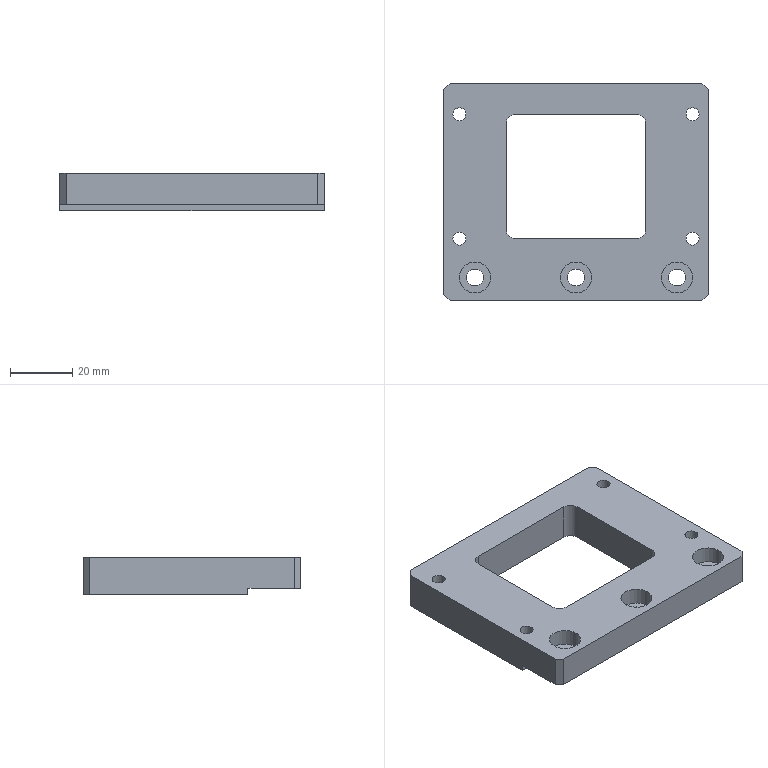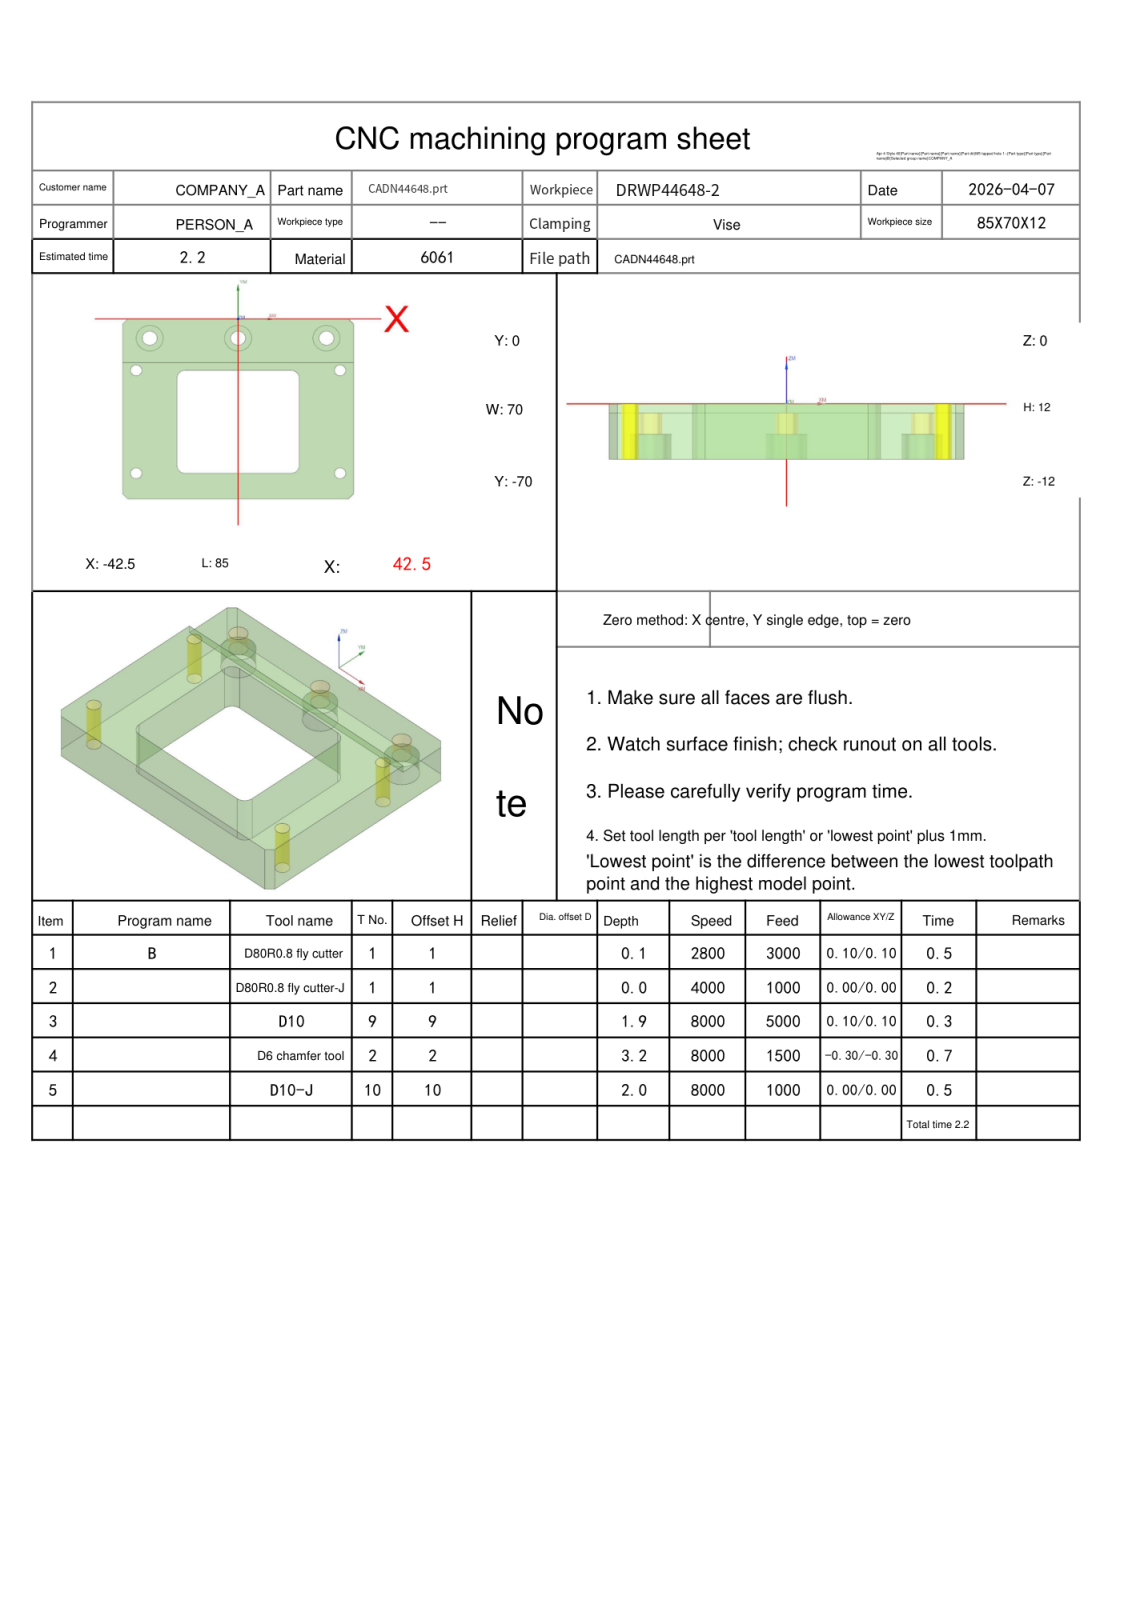NC program | NX | posted by the shop | part box 85 x 70 x 12 mm
Whole program:
%
O0001
(Machine time: 3.09 MIN)
(===Total Tool:4===)
(T1=D80R0.8 fly cutter D=80.  R=0.8  D-  H01 Z=0.    )
(T9=D10     D=10.  R=0.   D-  H09 Z=-1.9  )
(T2=D6 chamfer tool   D=6.   R=0.   D-  H02 Z=-3.2  )
(T10=D10-J  D=10.  R=0.   D10 H10 Z=-2.   )
G80 G90 G17 G49 G40
G91 G28 Z0
M01
N1 T01 M06
(D80R0.8 fly cutter  D=80. R=0.8 H=01 ce=0.10 di=0.10)
G00 G90 G54 X94.597 Y-35. M03 S2800
G43 H01 Z20.
M08
Z4.517
G01 Z2.517 F3000.
X82.597
X-82.597
X-94.597
Z4.517
G00 X94.597
Z4.033
G01 Z2.033
X82.597
X-82.597
X-94.597
Z4.033
G00 X94.597
Z3.55
G01 Z1.55
X82.597
X-82.597
X-94.597
Z3.55
G00 X94.597
Z3.067
G01 Z1.067
X82.597
X-82.597
X-94.597
Z3.067
G00 Z20.
X94.597
Z2.583
G01 Z.583
X82.597
X-82.597
X-94.597
Z2.583
G00 Z20.
X94.597
Z2.1
G01 Z.1
X82.597
X-82.597
X-94.597
Z2.1
G00 Z20.
G91 G28 Z0.0
M05
M09
G91 G28 Z0.0
M01
N2 T01 M06
(D80R0.8 fly cutter-J  D=80. R=0.8 H=01 ce=0.00 di=0.00)
G00 G90 G54 X94.499 Y-35. M03 S4000
G43 H01 Z20.
M08
Z2.
G01 Z0.0 F1000.
X82.499
X-82.499
X-94.499
Z2.
G00 Z20.
G91 G28 Z0.0
M05
M09
G91 G28 Z0.0
M01
N3 T09 M06
(D10  D=10. R=0. H=09 ce=0.10 di=0.10)
G00 G90 G54 X-48.714 Y3.1 M03 S8000
G43 H09 Z12.8
M08
Z1.025
G01 Z-.475 F5000.
X-44.33
X43.916
G02 X44.622 Y2.808 I-.001 J-1.
G01 X47.107 Y.322
G02 X47.4 Y-.384 I-.707 J-.707
G01 Y-3.401
G02 X46.401 Y-4.4 I-1. J.001
G01 X-46.544
G03 X-47.532 Y-5.245 I.001 J-1.
G01 X-48.388 Y-10.746
X-48.4 Y-10.9
G03 X-47.4 Y-11.9 I1. J0.0
G01 X47.4
X50.6
Z1.025
G00 X-48.714 Y3.1
Z.55
G01 Z-.95
X-44.33
X43.916
G02 X44.622 Y2.808 I-.001 J-1.
G01 X47.107 Y.322
G02 X47.4 Y-.384 I-.707 J-.707
G01 Y-3.401
G02 X46.401 Y-4.4 I-1. J.001
G01 X-46.544
G03 X-47.532 Y-5.245 I.001 J-1.
G01 X-48.388 Y-10.746
X-48.4 Y-10.9
G03 X-47.4 Y-11.9 I1. J0.0
G01 X47.4
X50.6
Z.55
G00 X-48.714 Y3.1
Z.075
G01 Z-1.425
X-44.33
X43.916
G02 X44.622 Y2.808 I-.001 J-1.
G01 X47.107 Y.322
G02 X47.4 Y-.384 I-.707 J-.707
G01 Y-3.401
G02 X46.401 Y-4.4 I-1. J.001
G01 X-46.544
G03 X-47.532 Y-5.245 I.001 J-1.
G01 X-48.388 Y-10.746
X-48.4 Y-10.9
G03 X-47.4 Y-11.9 I1. J0.0
G01 X47.4
X50.6
Z.075
G00 X-48.714 Y3.1
Z-.4
G01 Z-1.9
X-44.33
X43.916
G02 X44.622 Y2.808 I-.001 J-1.
G01 X47.107 Y.322
G02 X47.4 Y-.384 I-.707 J-.707
G01 Y-3.401
G02 X46.401 Y-4.4 I-1. J.001
G01 X-46.544
G03 X-47.532 Y-5.245 I.001 J-1.
G01 X-48.388 Y-10.746
X-48.4 Y-10.9
G03 X-47.4 Y-11.9 I1. J0.0
G01 X47.4
X50.6
Z-.4
G00 Z12.8
G91 G28 Z0.0
M05
M09
G91 G28 Z0.0
M01
N4 T02 M06
(D6 chamfer tool  D=6. R=0. H=02 ce=0.00 di=0.10)
G00 G90 G54 X-37.5 Y-20. M03 S8000
G43 H02 Z20.
M08
G98 G81 X-37.5 Y-20. Z-2.7 R3. F1000.
Y-60.
X37.5
Y-20.
G80
G00 Z20.
G00 G90 X-13.499 Y-20.7 M03 S7000
Z20.
Z2.5
G01 X-19.618 Z.273 F1500.
X-19.923 Y-20.736 Z.161
X-20.22 Y-20.813 Z.049
X-20.505 Y-20.928 Z-.063
X-20.772 Y-21.08 Z-.174
X-21.016 Y-21.267 Z-.286
X-21.233 Y-21.484 Z-.398
X-21.42 Y-21.728 Z-.51
X-21.572 Y-21.995 Z-.622
X-21.687 Y-22.28 Z-.734
X-21.764 Y-22.577 Z-.845
X-21.8 Y-22.882 Z-.957
Y-23. Z-1.
Y-57.
G03 X-19.5 Y-59.3 I2.3 J0.0
G01 X19.5
G03 X21.8 Y-57. I0.0 J2.3
G01 Y-23.
G03 X19.5 Y-20.7 I-2.3 J0.0
G01 X-19.5
G03 X-21.8 Y-23. I0.0 J-2.3
G01 Y-23.5
Z1.5
G00 Z20.
G00 G90 X-.386 Y-15.773 M03 S6500
Z20.
Z.172
G01 Z-1.2 F1500.
G03 X-.1 Y-15.973 I1.286 J1.532
G01 X-.054 Y-16.003
X0.0 Y-16.
X42.5
G02 X43.5 Y-17. I0.0 J-1.
G01 Y-68.
X43.466 Y-68.259
X43.366 Y-68.5
X43.207 Y-68.707
X41.207 Y-70.707
X41. Y-70.866
X40.759 Y-70.966
X40.5 Y-71.
X-40.5
X-40.759 Y-70.966
X-41. Y-70.866
X-41.207 Y-70.707
X-43.207 Y-68.707
X-43.366 Y-68.5
X-43.466 Y-68.259
X-43.5 Y-68.
Y-17.
G02 X-42.5 Y-16. I1. J0.0
G01 X0.0
X.054 Y-16.003
X.1 Y-15.973
G03 X.386 Y-15.773 I-1. J1.732
G01 Z.172
G00 Z10.
X-38.426 Y-19.588
Z.32
G01 Z-1.2
G03 X-38.586 Y-19.897 I1.687 J-1.075
G01 X-38.61 Y-19.946
X-38.6 Y-20.
G03 X-37.5 Y-21.1 I1.1 J0.0
X-36.4 Y-20. I0.0 J1.1
X-37.5 Y-18.9 I-1.1 J0.0
X-38.6 Y-20. I0.0 J-1.1
G01 X-38.61 Y-20.054
X-38.586 Y-20.103
G03 X-38.426 Y-20.412 I1.848 J.765
G01 Z.32
G00 Z10.
Y-59.588
Z.32
G01 Z-1.2
G03 X-38.586 Y-59.897 I1.687 J-1.075
G01 X-38.61 Y-59.946
X-38.6 Y-60.
G03 X-37.5 Y-61.1 I1.1 J0.0
X-36.4 Y-60. I0.0 J1.1
X-37.5 Y-58.9 I-1.1 J0.0
X-38.6 Y-60. I0.0 J-1.1
G01 X-38.61 Y-60.054
X-38.586 Y-60.103
G03 X-38.426 Y-60.412 I1.848 J.765
G01 Z.32
G00 Z10.
X21.273 Y-40.386
Z.172
G01 Z-1.2
G03 X21.473 Y-40.1 I-1.532 J1.286
G01 X21.503 Y-40.054
X21.5 Y-40.
Y-23.
G03 X19.5 Y-21. I-2. J0.0
G01 X-19.5
G03 X-21.5 Y-23. I0.0 J-2.
G01 Y-57.
G03 X-19.5 Y-59. I2. J0.0
G01 X19.5
G03 X21.5 Y-57. I0.0 J2.
G01 Y-40.
X21.503 Y-39.946
X21.473 Y-39.9
G03 X21.273 Y-39.614 I-1.732 J-1.
G01 Z.172
G00 Z10.
X36.574 Y-59.588
Z.32
G01 Z-1.2
G03 X36.414 Y-59.897 I1.687 J-1.075
G01 X36.39 Y-59.946
X36.4 Y-60.
G03 X37.5 Y-61.1 I1.1 J0.0
X38.6 Y-60. I0.0 J1.1
X37.5 Y-58.9 I-1.1 J0.0
X36.4 Y-60. I0.0 J-1.1
G01 X36.39 Y-60.054
X36.414 Y-60.103
G03 X36.574 Y-60.412 I1.848 J.765
G01 Z.32
G00 Z10.
Y-19.588
Z.32
G01 Z-1.2
G03 X36.414 Y-19.897 I1.687 J-1.075
G01 X36.39 Y-19.946
X36.4 Y-20.
G03 X37.5 Y-21.1 I1.1 J0.0
X38.6 Y-20. I0.0 J1.1
X37.5 Y-18.9 I-1.1 J0.0
X36.4 Y-20. I0.0 J-1.1
G01 X36.39 Y-20.054
X36.414 Y-20.103
G03 X36.574 Y-20.412 I1.848 J.765
G01 Z.32
G00 Z10.
X-43.568 Y-14.01
Z-1.669
G01 Z-3.2
X-43.508 Y-13.925
X-43.5 Y-13.895
Y-2.
X-43.466 Y-1.741
X-43.366 Y-1.5
X-43.207 Y-1.293
X-41.207 Y.707
X-41. Y.866
X-40.759 Y.966
X-40.5 Y1.
X40.5
X40.759 Y.966
X41. Y.866
X41.207 Y.707
X43.207 Y-1.293
X43.366 Y-1.5
X43.466 Y-1.741
X43.5 Y-2.
Y-13.895
X43.508 Y-13.925
X43.568 Y-14.01
Z-1.669
G00 Z10.
X30.935 Y-7.093
Z-1.73
G01 Z-3.2
G03 X30.766 Y-7.398 I1.658 J-1.118
G01 X30.741 Y-7.446
X30.75 Y-7.5
G03 X32.5 Y-9.25 I1.75 J0.0
X34.25 Y-7.5 I0.0 J1.75
X32.5 Y-5.75 I-1.75 J0.0
X30.75 Y-7.5 I0.0 J-1.75
G01 X30.741 Y-7.554
X30.766 Y-7.602
G03 X30.935 Y-7.907 I1.827 J.813
G01 Z-1.73
G00 Z10.
X-1.565 Y-7.093
Z-1.73
G01 Z-3.2
G03 X-1.734 Y-7.398 I1.658 J-1.118
G01 X-1.759 Y-7.446
X-1.75 Y-7.5
G03 X0.0 Y-9.25 I1.75 J0.0
X1.75 Y-7.5 I0.0 J1.75
X0.0 Y-5.75 I-1.75 J0.0
X-1.75 Y-7.5 I0.0 J-1.75
G01 X-1.759 Y-7.554
X-1.734 Y-7.602
G03 X-1.565 Y-7.907 I1.827 J.813
G01 Z-1.73
G00 Z10.
X-34.065 Y-7.093
Z-1.73
G01 Z-3.2
G03 X-34.234 Y-7.398 I1.658 J-1.118
G01 X-34.259 Y-7.446
X-34.25 Y-7.5
G03 X-32.5 Y-9.25 I1.75 J0.0
X-30.75 Y-7.5 I0.0 J1.75
X-32.5 Y-5.75 I-1.75 J0.0
X-34.25 Y-7.5 I0.0 J-1.75
G01 X-34.259 Y-7.554
X-34.234 Y-7.602
G03 X-34.065 Y-7.907 I1.827 J.813
G01 Z-1.73
G00 Z20.
G91 G28 Z0.0
M05
M09
G91 G28 Z0.0
M01
N5 T10 M06
(D10-J  D=10. R=0. H=10 ce=0.40 di=0.00)
G00 G90 G54 X-48.337 Y2.062 M03 S8000
G43 H10 Z12.8
M08
Z-.5
G01 Z-2. F1000.
G03 X-46.571 Y1. I1.766 J.938
G01 X46.158
G02 X46.863 Y.708 I-.001 J-1.
G01 X47.207 Y.364
G02 X47.5 Y-.343 I-.707 J-.707
G01 Y-2.201
G02 X46.501 Y-3.2 I-1. J.001
G01 X-46.6
G03 X-47.5 Y-4.1 I0.0 J-.9
G01 Y-6.4
G03 X-46.5 Y-7.4 I1. J0.0
G01 X46.6
G02 X47.5 Y-8.3 I0.0 J-.9
G01 Y-10.6
G02 X46.5 Y-11.6 I-1. J0.0
G01 X-47.5
G02 X-49.5 Y-9.6 I0.0 J2.
G01 Z-.5
G00 Z12.8
G00 G90 X-49.5 Y-9.801 M03 S8000
Z12.8
Z-1.
G01 Z-2. F1000.
G41 D10
Y-10.001
G03 X-47.5 Y-12. I2. J.001
G01 X47.5
G03 X49.5 Y-10.001 I0.0 J2.
G01 G40 Y-9.801
Z-1.
G00 Z12.8
M05
M09
G91 G28 Z0.0
G91 G28 Y0.0
M30
%